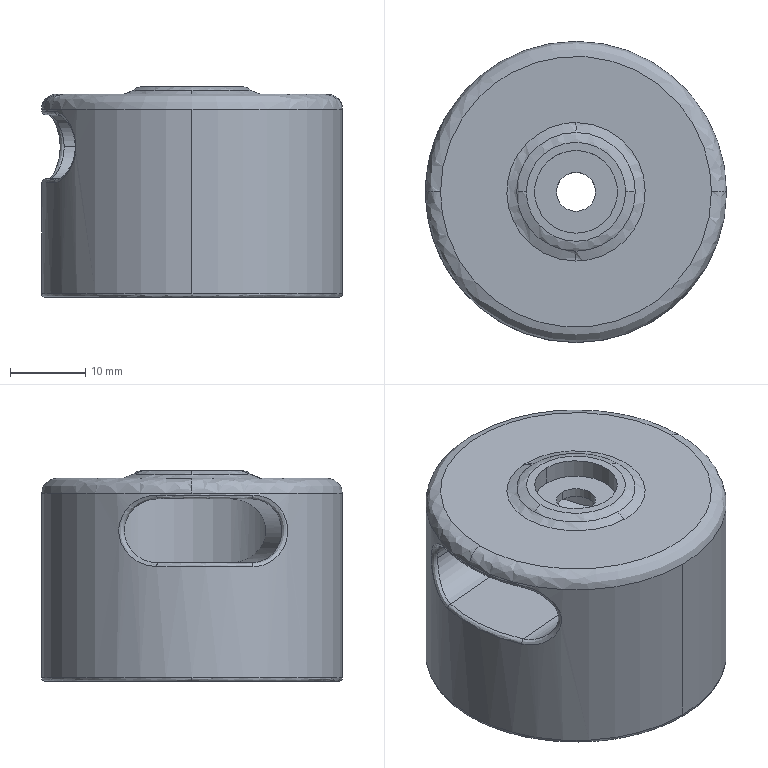Part | SolidWorks | features BaseBody 1 | 1 solid | 97 faces | box 40 x 40 x 27.99 mm | volume 18357 mm3 | plane 44 | cylinder 41 | spline 12 | commonest cylinder face diameters 10.2 x5 13.1 x5 20.757 x5 23.157 x5 5.2 x4 8.5 x3